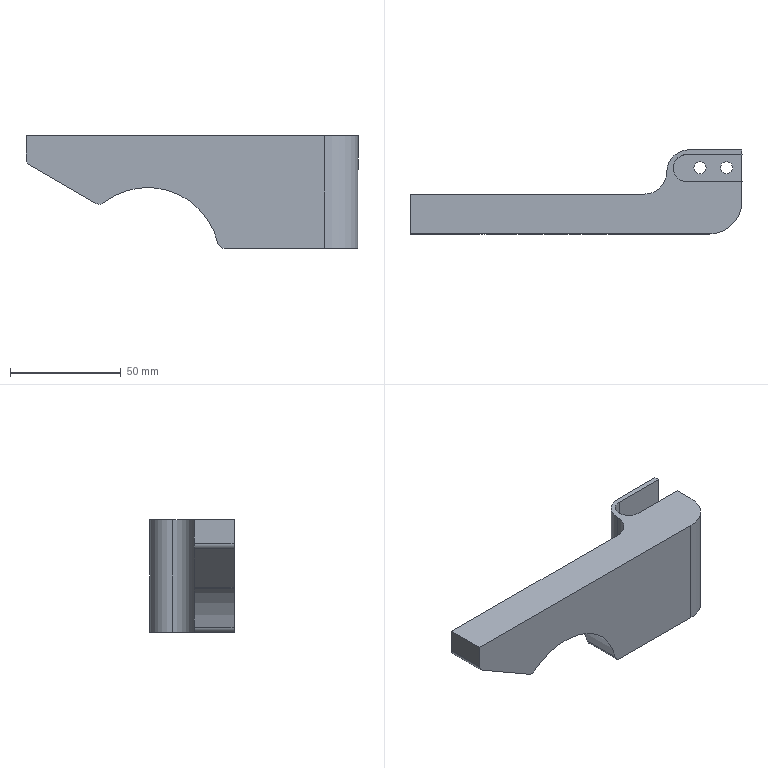Part | NX | 1 solid | 25 faces | box 150 x 38 x 51 mm | volume 119385 mm3 | plane 13 | cylinder 12 | commonest cylinder face diameters 6 x3 5.5 x2 11.5 x2 20 x2 12.2 x1 30 x1
STEP:
#1=CARTESIAN_POINT('',(75.,16.87,0.));
#2=VERTEX_POINT('',#1);
#3=CARTESIAN_POINT('',(50.,16.87,0.));
#4=VERTEX_POINT('',#3);
#5=CARTESIAN_POINT('',(75.,16.87,0.));
#6=DIRECTION('',(-1.,0.,0.));
#7=VECTOR('',#6,1000.);
#8=LINE('',#5,#7);
#9=EDGE_CURVE('',#2,#4,#8,.T.);
#10=ORIENTED_EDGE('',*,*,#9,.F.);
#11=CARTESIAN_POINT('',(75.,19.,0.));
#12=VERTEX_POINT('',#11);
#13=CARTESIAN_POINT('',(75.,-31.,0.));
#14=DIRECTION('',(0.,1.,0.));
#15=VECTOR('',#14,1000.);
#16=LINE('',#13,#15);
#17=EDGE_CURVE('',#2,#12,#16,.T.);
#18=ORIENTED_EDGE('',*,*,#17,.T.);
#19=CARTESIAN_POINT('',(51.,19.,0.));
#20=VERTEX_POINT('',#19);
#21=CARTESIAN_POINT('',(75.,19.,0.));
#22=DIRECTION('',(-1.,0.,0.));
#23=VECTOR('',#22,1000.);
#24=LINE('',#21,#23);
#25=EDGE_CURVE('',#12,#20,#24,.T.);
#26=ORIENTED_EDGE('',*,*,#25,.T.);
#27=CARTESIAN_POINT('',(41.,9.,0.));
#28=VERTEX_POINT('',#27);
#29=CARTESIAN_POINT('',(51.,9.,0.));
#30=DIRECTION('',(0.,0.,1.));
#31=DIRECTION('',(1.,0.,0.));
#32=AXIS2_PLACEMENT_3D('',#29,#30,#31);
#33=CIRCLE('',#32,10.);
#34=EDGE_CURVE('',#20,#28,#33,.T.);
#35=ORIENTED_EDGE('',*,*,#34,.T.);
#36=CARTESIAN_POINT('',(31.,-1.,0.));
#37=VERTEX_POINT('',#36);
#38=CARTESIAN_POINT('',(31.,9.,0.));
#39=DIRECTION('',(0.,0.,-1.));
#40=DIRECTION('',(0.,1.,0.));
#41=AXIS2_PLACEMENT_3D('',#38,#39,#40);
#42=CIRCLE('',#41,10.);
#43=EDGE_CURVE('',#28,#37,#42,.T.);
#44=ORIENTED_EDGE('',*,*,#43,.T.);
#45=CARTESIAN_POINT('',(-75.,-1.,0.));
#46=VERTEX_POINT('',#45);
#47=CARTESIAN_POINT('',(31.,-1.,0.));
#48=DIRECTION('',(-1.,0.,0.));
#49=VECTOR('',#48,1000.);
#50=LINE('',#47,#49);
#51=EDGE_CURVE('',#37,#46,#50,.T.);
#52=ORIENTED_EDGE('',*,*,#51,.T.);
#53=CARTESIAN_POINT('',(-75.,-19.,0.));
#54=VERTEX_POINT('',#53);
#55=CARTESIAN_POINT('',(-75.,-31.,0.));
#56=DIRECTION('',(0.,1.,0.));
#57=VECTOR('',#56,1000.);
#58=LINE('',#55,#57);
#59=EDGE_CURVE('',#46,#54,#58,.F.);
#60=ORIENTED_EDGE('',*,*,#59,.T.);
#61=CARTESIAN_POINT('',(60.,-19.,0.));
#62=VERTEX_POINT('',#61);
#63=CARTESIAN_POINT('',(-75.,-19.,0.));
#64=DIRECTION('',(1.,0.,0.));
#65=VECTOR('',#64,1000.);
#66=LINE('',#63,#65);
#67=EDGE_CURVE('',#54,#62,#66,.T.);
#68=ORIENTED_EDGE('',*,*,#67,.T.);
#69=CARTESIAN_POINT('',(75.,-4.,0.));
#70=VERTEX_POINT('',#69);
#71=CARTESIAN_POINT('',(60.,-4.,0.));
#72=DIRECTION('',(0.,0.,1.));
#73=DIRECTION('',(1.,0.,0.));
#74=AXIS2_PLACEMENT_3D('',#71,#72,#73);
#75=CIRCLE('',#74,15.);
#76=EDGE_CURVE('',#62,#70,#75,.T.);
#77=ORIENTED_EDGE('',*,*,#76,.T.);
#78=CARTESIAN_POINT('',(75.,4.67,0.));
#79=VERTEX_POINT('',#78);
#80=CARTESIAN_POINT('',(75.,-31.,0.));
#81=DIRECTION('',(0.,1.,0.));
#82=VECTOR('',#81,1000.);
#83=LINE('',#80,#82);
#84=EDGE_CURVE('',#70,#79,#83,.T.);
#85=ORIENTED_EDGE('',*,*,#84,.T.);
#86=CARTESIAN_POINT('',(50.,4.67,0.));
#87=VERTEX_POINT('',#86);
#88=CARTESIAN_POINT('',(50.,4.67,0.));
#89=DIRECTION('',(1.,0.,0.));
#90=VECTOR('',#89,1000.);
#91=LINE('',#88,#90);
#92=EDGE_CURVE('',#87,#79,#91,.T.);
#93=ORIENTED_EDGE('',*,*,#92,.F.);
#94=CARTESIAN_POINT('',(50.,10.77,0.));
#95=DIRECTION('',(0.,0.,1.));
#96=DIRECTION('',(1.,0.,0.));
#97=AXIS2_PLACEMENT_3D('',#94,#95,#96);
#98=CIRCLE('',#97,6.1);
#99=EDGE_CURVE('',#4,#87,#98,.T.);
#100=ORIENTED_EDGE('',*,*,#99,.F.);
#101=EDGE_LOOP('',(#10,#18,#26,#35,#44,#52,#60,#68,#77,#85,#93,#100));
#102=FACE_BOUND('',#101,.T.);
#103=CARTESIAN_POINT('',(75.,-31.,0.));
#104=DIRECTION('',(0.,0.,-1.));
#105=DIRECTION('',(0.,1.,0.));
#106=AXIS2_PLACEMENT_3D('',#103,#104,#105);
#107=PLANE('',#106);
#108=ADVANCED_FACE('',(#102),#107,.F.);
#109=CARTESIAN_POINT('',(70.75,10.9,-25.2));
#110=VERTEX_POINT('',#109);
#111=CARTESIAN_POINT('',(68.,10.9,-25.2));
#112=DIRECTION('',(0.,0.,-1.));
#113=DIRECTION('',(1.,0.,0.));
#114=AXIS2_PLACEMENT_3D('',#111,#112,#113);
#115=CIRCLE('',#114,2.75);
#116=EDGE_CURVE('',#110,#110,#115,.F.);
#117=ORIENTED_EDGE('',*,*,#116,.F.);
#118=EDGE_LOOP('',(#117));
#119=FACE_BOUND('',#118,.T.);
#120=CARTESIAN_POINT('',(70.75,10.9,-15.2));
#121=VERTEX_POINT('',#120);
#122=CARTESIAN_POINT('',(68.,10.9,-15.2));
#123=DIRECTION('',(0.,0.,1.));
#124=DIRECTION('',(1.,0.,0.));
#125=AXIS2_PLACEMENT_3D('',#122,#123,#124);
#126=CIRCLE('',#125,2.75);
#127=EDGE_CURVE('',#121,#121,#126,.F.);
#128=ORIENTED_EDGE('',*,*,#127,.F.);
#129=EDGE_LOOP('',(#128));
#130=FACE_BOUND('',#129,.T.);
#131=CARTESIAN_POINT('',(68.,10.9,0.));
#132=DIRECTION('',(0.,0.,-1.));
#133=DIRECTION('',(1.,0.,0.));
#134=AXIS2_PLACEMENT_3D('',#131,#132,#133);
#135=CYLINDRICAL_SURFACE('',#134,2.75);
#136=ADVANCED_FACE('',(#119,#130),#135,.F.);
#137=CARTESIAN_POINT('',(58.75,10.9,-25.2));
#138=VERTEX_POINT('',#137);
#139=CARTESIAN_POINT('',(56.,10.9,-25.2));
#140=DIRECTION('',(0.,0.,-1.));
#141=DIRECTION('',(1.,0.,0.));
#142=AXIS2_PLACEMENT_3D('',#139,#140,#141);
#143=CIRCLE('',#142,2.75);
#144=EDGE_CURVE('',#138,#138,#143,.F.);
#145=ORIENTED_EDGE('',*,*,#144,.F.);
#146=EDGE_LOOP('',(#145));
#147=FACE_BOUND('',#146,.T.);
#148=CARTESIAN_POINT('',(58.75,10.9,-15.2));
#149=VERTEX_POINT('',#148);
#150=CARTESIAN_POINT('',(56.,10.9,-15.2));
#151=DIRECTION('',(0.,0.,1.));
#152=DIRECTION('',(1.,0.,0.));
#153=AXIS2_PLACEMENT_3D('',#150,#151,#152);
#154=CIRCLE('',#153,2.75);
#155=EDGE_CURVE('',#149,#149,#154,.F.);
#156=ORIENTED_EDGE('',*,*,#155,.F.);
#157=EDGE_LOOP('',(#156));
#158=FACE_BOUND('',#157,.T.);
#159=CARTESIAN_POINT('',(56.,10.9,0.));
#160=DIRECTION('',(0.,0.,-1.));
#161=DIRECTION('',(1.,0.,0.));
#162=AXIS2_PLACEMENT_3D('',#159,#160,#161);
#163=CYLINDRICAL_SURFACE('',#162,2.75);
#164=ADVANCED_FACE('',(#147,#158),#163,.F.);
#165=CARTESIAN_POINT('',(-73.5,-19.,-13.246));
#166=VERTEX_POINT('',#165);
#167=CARTESIAN_POINT('',(-73.5,-1.,-13.246));
#168=VERTEX_POINT('',#167);
#169=CARTESIAN_POINT('',(-73.5,-31.,-13.246));
#170=DIRECTION('',(0.,1.,0.));
#171=VECTOR('',#170,1000.);
#172=LINE('',#169,#171);
#173=EDGE_CURVE('',#166,#168,#172,.T.);
#174=ORIENTED_EDGE('',*,*,#173,.F.);
#175=CARTESIAN_POINT('',(-75.,-19.,-10.648));
#176=VERTEX_POINT('',#175);
#177=CARTESIAN_POINT('',(-72.,-19.,-10.648));
#178=DIRECTION('',(0.,1.,0.));
#179=DIRECTION('',(1.,0.,0.));
#180=AXIS2_PLACEMENT_3D('',#177,#178,#179);
#181=CIRCLE('',#180,3.);
#182=EDGE_CURVE('',#166,#176,#181,.T.);
#183=ORIENTED_EDGE('',*,*,#182,.T.);
#184=CARTESIAN_POINT('',(-75.,-1.,-10.648));
#185=VERTEX_POINT('',#184);
#186=CARTESIAN_POINT('',(-75.,-31.,-10.648));
#187=DIRECTION('',(0.,1.,0.));
#188=VECTOR('',#187,1000.);
#189=LINE('',#186,#188);
#190=EDGE_CURVE('',#176,#185,#189,.T.);
#191=ORIENTED_EDGE('',*,*,#190,.T.);
#192=CARTESIAN_POINT('',(-72.,-1.,-10.648));
#193=DIRECTION('',(0.,-1.,0.));
#194=DIRECTION('',(-1.,0.,0.));
#195=AXIS2_PLACEMENT_3D('',#192,#193,#194);
#196=CIRCLE('',#195,3.);
#197=EDGE_CURVE('',#185,#168,#196,.T.);
#198=ORIENTED_EDGE('',*,*,#197,.T.);
#199=EDGE_LOOP('',(#174,#183,#191,#198));
#200=FACE_BOUND('',#199,.T.);
#201=CARTESIAN_POINT('',(-72.,-31.,-10.648));
#202=DIRECTION('',(0.,1.,0.));
#203=DIRECTION('',(1.,0.,0.));
#204=AXIS2_PLACEMENT_3D('',#201,#202,#203);
#205=CYLINDRICAL_SURFACE('',#204,3.);
#206=ADVANCED_FACE('',(#200),#205,.T.);
#207=CARTESIAN_POINT('',(-43.38,-19.,-30.636));
#208=VERTEX_POINT('',#207);
#209=CARTESIAN_POINT('',(-43.38,-1.,-30.636));
#210=VERTEX_POINT('',#209);
#211=CARTESIAN_POINT('',(-43.38,-31.,-30.636));
#212=DIRECTION('',(0.,1.,0.));
#213=VECTOR('',#212,1000.);
#214=LINE('',#211,#213);
#215=EDGE_CURVE('',#208,#210,#214,.T.);
#216=ORIENTED_EDGE('',*,*,#215,.F.);
#217=CARTESIAN_POINT('',(-73.5,-19.,-13.246));
#218=DIRECTION('',(-0.866,0.,0.5));
#219=VECTOR('',#218,1000.);
#220=LINE('',#217,#219);
#221=EDGE_CURVE('',#208,#166,#220,.T.);
#222=ORIENTED_EDGE('',*,*,#221,.T.);
#223=ORIENTED_EDGE('',*,*,#173,.T.);
#224=CARTESIAN_POINT('',(-73.5,-1.,-13.246));
#225=DIRECTION('',(0.866,0.,-0.5));
#226=VECTOR('',#225,1000.);
#227=LINE('',#224,#226);
#228=EDGE_CURVE('',#168,#210,#227,.T.);
#229=ORIENTED_EDGE('',*,*,#228,.T.);
#230=EDGE_LOOP('',(#216,#222,#223,#229));
#231=FACE_BOUND('',#230,.T.);
#232=CARTESIAN_POINT('',(-73.5,-31.,-13.246));
#233=DIRECTION('',(0.5,0.,0.866));
#234=DIRECTION('',(0.866,0.,-0.5));
#235=AXIS2_PLACEMENT_3D('',#232,#233,#234);
#236=PLANE('',#235);
#237=ADVANCED_FACE('',(#231),#236,.F.);
#238=CARTESIAN_POINT('',(-40.031,-19.,-30.401));
#239=VERTEX_POINT('',#238);
#240=CARTESIAN_POINT('',(-40.031,-1.,-30.401));
#241=VERTEX_POINT('',#240);
#242=CARTESIAN_POINT('',(-40.031,-31.,-30.401));
#243=DIRECTION('',(0.,1.,0.));
#244=VECTOR('',#243,1000.);
#245=LINE('',#242,#244);
#246=EDGE_CURVE('',#239,#241,#245,.T.);
#247=ORIENTED_EDGE('',*,*,#246,.F.);
#248=CARTESIAN_POINT('',(-41.88,-19.,-28.038));
#249=DIRECTION('',(0.,1.,0.));
#250=DIRECTION('',(1.,0.,0.));
#251=AXIS2_PLACEMENT_3D('',#248,#249,#250);
#252=CIRCLE('',#251,3.);
#253=EDGE_CURVE('',#239,#208,#252,.T.);
#254=ORIENTED_EDGE('',*,*,#253,.T.);
#255=ORIENTED_EDGE('',*,*,#215,.T.);
#256=CARTESIAN_POINT('',(-41.88,-1.,-28.038));
#257=DIRECTION('',(0.,-1.,0.));
#258=DIRECTION('',(-1.,0.,0.));
#259=AXIS2_PLACEMENT_3D('',#256,#257,#258);
#260=CIRCLE('',#259,3.);
#261=EDGE_CURVE('',#210,#241,#260,.T.);
#262=ORIENTED_EDGE('',*,*,#261,.T.);
#263=EDGE_LOOP('',(#247,#254,#255,#262));
#264=FACE_BOUND('',#263,.T.);
#265=CARTESIAN_POINT('',(-41.88,-31.,-28.038));
#266=DIRECTION('',(0.,1.,0.));
#267=DIRECTION('',(1.,0.,0.));
#268=AXIS2_PLACEMENT_3D('',#265,#266,#267);
#269=CYLINDRICAL_SURFACE('',#268,3.);
#270=ADVANCED_FACE('',(#264),#269,.T.);
#271=CARTESIAN_POINT('',(11.66,-19.,-48.676));
#272=VERTEX_POINT('',#271);
#273=CARTESIAN_POINT('',(11.66,-1.,-48.676));
#274=VERTEX_POINT('',#273);
#275=CARTESIAN_POINT('',(11.66,-31.,-48.676));
#276=DIRECTION('',(0.,1.,0.));
#277=VECTOR('',#276,1000.);
#278=LINE('',#275,#277);
#279=EDGE_CURVE('',#272,#274,#278,.T.);
#280=ORIENTED_EDGE('',*,*,#279,.F.);
#281=CARTESIAN_POINT('',(-20.005,-19.,-55.997));
#282=DIRECTION('',(0.,1.,0.));
#283=DIRECTION('',(1.,0.,0.));
#284=AXIS2_PLACEMENT_3D('',#281,#282,#283);
#285=CIRCLE('',#284,32.5);
#286=EDGE_CURVE('',#272,#239,#285,.F.);
#287=ORIENTED_EDGE('',*,*,#286,.T.);
#288=ORIENTED_EDGE('',*,*,#246,.T.);
#289=CARTESIAN_POINT('',(-20.005,-1.,-55.997));
#290=DIRECTION('',(0.,-1.,0.));
#291=DIRECTION('',(-1.,0.,0.));
#292=AXIS2_PLACEMENT_3D('',#289,#290,#291);
#293=CIRCLE('',#292,32.5);
#294=EDGE_CURVE('',#241,#274,#293,.F.);
#295=ORIENTED_EDGE('',*,*,#294,.T.);
#296=EDGE_LOOP('',(#280,#287,#288,#295));
#297=FACE_BOUND('',#296,.T.);
#298=CARTESIAN_POINT('',(-20.005,-31.,-55.997));
#299=DIRECTION('',(0.,1.,0.));
#300=DIRECTION('',(1.,0.,0.));
#301=AXIS2_PLACEMENT_3D('',#298,#299,#300);
#302=CYLINDRICAL_SURFACE('',#301,32.5);
#303=ADVANCED_FACE('',(#297),#302,.F.);
#304=CARTESIAN_POINT('',(14.583,-19.,-51.));
#305=VERTEX_POINT('',#304);
#306=CARTESIAN_POINT('',(14.583,-1.,-51.));
#307=VERTEX_POINT('',#306);
#308=CARTESIAN_POINT('',(14.583,-31.,-51.));
#309=DIRECTION('',(0.,1.,0.));
#310=VECTOR('',#309,1000.);
#311=LINE('',#308,#310);
#312=EDGE_CURVE('',#305,#307,#311,.T.);
#313=ORIENTED_EDGE('',*,*,#312,.F.);
#314=CARTESIAN_POINT('',(14.583,-19.,-48.));
#315=DIRECTION('',(0.,1.,0.));
#316=DIRECTION('',(1.,0.,0.));
#317=AXIS2_PLACEMENT_3D('',#314,#315,#316);
#318=CIRCLE('',#317,3.);
#319=EDGE_CURVE('',#305,#272,#318,.T.);
#320=ORIENTED_EDGE('',*,*,#319,.T.);
#321=ORIENTED_EDGE('',*,*,#279,.T.);
#322=CARTESIAN_POINT('',(14.583,-1.,-48.));
#323=DIRECTION('',(0.,-1.,0.));
#324=DIRECTION('',(-1.,0.,0.));
#325=AXIS2_PLACEMENT_3D('',#322,#323,#324);
#326=CIRCLE('',#325,3.);
#327=EDGE_CURVE('',#274,#307,#326,.T.);
#328=ORIENTED_EDGE('',*,*,#327,.T.);
#329=EDGE_LOOP('',(#313,#320,#321,#328));
#330=FACE_BOUND('',#329,.T.);
#331=CARTESIAN_POINT('',(14.583,-31.,-48.));
#332=DIRECTION('',(0.,1.,0.));
#333=DIRECTION('',(1.,0.,0.));
#334=AXIS2_PLACEMENT_3D('',#331,#332,#333);
#335=CYLINDRICAL_SURFACE('',#334,3.);
#336=ADVANCED_FACE('',(#330),#335,.T.);
#337=CARTESIAN_POINT('',(51.,19.,-51.));
#338=VERTEX_POINT('',#337);
#339=CARTESIAN_POINT('',(41.,9.,-51.));
#340=VERTEX_POINT('',#339);
#341=CARTESIAN_POINT('',(51.,9.,-51.));
#342=DIRECTION('',(0.,0.,1.));
#343=DIRECTION('',(1.,0.,0.));
#344=AXIS2_PLACEMENT_3D('',#341,#342,#343);
#345=CIRCLE('',#344,10.);
#346=EDGE_CURVE('',#338,#340,#345,.T.);
#347=ORIENTED_EDGE('',*,*,#346,.T.);
#348=CARTESIAN_POINT('',(41.,9.,0.));
#349=DIRECTION('',(0.,0.,-1.));
#350=VECTOR('',#349,1000.);
#351=LINE('',#348,#350);
#352=EDGE_CURVE('',#28,#340,#351,.T.);
#353=ORIENTED_EDGE('',*,*,#352,.F.);
#354=ORIENTED_EDGE('',*,*,#34,.F.);
#355=CARTESIAN_POINT('',(51.,19.,0.));
#356=DIRECTION('',(0.,0.,-1.));
#357=VECTOR('',#356,1000.);
#358=LINE('',#355,#357);
#359=EDGE_CURVE('',#20,#338,#358,.T.);
#360=ORIENTED_EDGE('',*,*,#359,.T.);
#361=EDGE_LOOP('',(#347,#353,#354,#360));
#362=FACE_BOUND('',#361,.T.);
#363=CARTESIAN_POINT('',(51.,9.,0.));
#364=DIRECTION('',(0.,0.,-1.));
#365=DIRECTION('',(1.,0.,0.));
#366=AXIS2_PLACEMENT_3D('',#363,#364,#365);
#367=CYLINDRICAL_SURFACE('',#366,10.);
#368=ADVANCED_FACE('',(#362),#367,.T.);
#369=ORIENTED_EDGE('',*,*,#197,.F.);
#370=CARTESIAN_POINT('',(-75.,-1.,0.));
#371=DIRECTION('',(0.,0.,-1.));
#372=VECTOR('',#371,1000.);
#373=LINE('',#370,#372);
#374=EDGE_CURVE('',#46,#185,#373,.T.);
#375=ORIENTED_EDGE('',*,*,#374,.F.);
#376=ORIENTED_EDGE('',*,*,#51,.F.);
#377=CARTESIAN_POINT('',(31.,-1.,-51.));
#378=VERTEX_POINT('',#377);
#379=CARTESIAN_POINT('',(31.,-1.,0.));
#380=DIRECTION('',(0.,0.,-1.));
#381=VECTOR('',#380,1000.);
#382=LINE('',#379,#381);
#383=EDGE_CURVE('',#37,#378,#382,.T.);
#384=ORIENTED_EDGE('',*,*,#383,.T.);
#385=CARTESIAN_POINT('',(31.,-1.,-51.));
#386=DIRECTION('',(-1.,0.,0.));
#387=VECTOR('',#386,1000.);
#388=LINE('',#385,#387);
#389=EDGE_CURVE('',#378,#307,#388,.T.);
#390=ORIENTED_EDGE('',*,*,#389,.T.);
#391=ORIENTED_EDGE('',*,*,#327,.F.);
#392=ORIENTED_EDGE('',*,*,#294,.F.);
#393=ORIENTED_EDGE('',*,*,#261,.F.);
#394=ORIENTED_EDGE('',*,*,#228,.F.);
#395=EDGE_LOOP('',(#369,#375,#376,#384,#390,#391,#392,#393,#394));
#396=FACE_BOUND('',#395,.T.);
#397=CARTESIAN_POINT('',(31.,-1.,0.));
#398=DIRECTION('',(0.,-1.,0.));
#399=DIRECTION('',(0.,0.,-1.));
#400=AXIS2_PLACEMENT_3D('',#397,#398,#399);
#401=PLANE('',#400);
#402=ADVANCED_FACE('',(#396),#401,.F.);
#403=CARTESIAN_POINT('',(31.,9.,-51.));
#404=DIRECTION('',(0.,0.,1.));
#405=DIRECTION('',(0.,-1.,0.));
#406=AXIS2_PLACEMENT_3D('',#403,#404,#405);
#407=CIRCLE('',#406,10.);
#408=EDGE_CURVE('',#340,#378,#407,.F.);
#409=ORIENTED_EDGE('',*,*,#408,.T.);
#410=ORIENTED_EDGE('',*,*,#383,.F.);
#411=ORIENTED_EDGE('',*,*,#43,.F.);
#412=ORIENTED_EDGE('',*,*,#352,.T.);
#413=EDGE_LOOP('',(#409,#410,#411,#412));
#414=FACE_BOUND('',#413,.T.);
#415=CARTESIAN_POINT('',(31.,9.,0.));
#416=DIRECTION('',(0.,0.,-1.));
#417=DIRECTION('',(1.,0.,0.));
#418=AXIS2_PLACEMENT_3D('',#415,#416,#417);
#419=CYLINDRICAL_SURFACE('',#418,10.);
#420=ADVANCED_FACE('',(#414),#419,.F.);
#421=CARTESIAN_POINT('',(60.,-19.,-51.));
#422=VERTEX_POINT('',#421);
#423=CARTESIAN_POINT('',(75.,-4.,-51.));
#424=VERTEX_POINT('',#423);
#425=CARTESIAN_POINT('',(60.,-4.,-51.));
#426=DIRECTION('',(0.,0.,1.));
#427=DIRECTION('',(1.,0.,0.));
#428=AXIS2_PLACEMENT_3D('',#425,#426,#427);
#429=CIRCLE('',#428,15.);
#430=EDGE_CURVE('',#422,#424,#429,.T.);
#431=ORIENTED_EDGE('',*,*,#430,.T.);
#432=CARTESIAN_POINT('',(75.,-4.,0.));
#433=DIRECTION('',(0.,0.,-1.));
#434=VECTOR('',#433,1000.);
#435=LINE('',#432,#434);
#436=EDGE_CURVE('',#70,#424,#435,.T.);
#437=ORIENTED_EDGE('',*,*,#436,.F.);
#438=ORIENTED_EDGE('',*,*,#76,.F.);
#439=CARTESIAN_POINT('',(60.,-19.,0.));
#440=DIRECTION('',(0.,0.,-1.));
#441=VECTOR('',#440,1000.);
#442=LINE('',#439,#441);
#443=EDGE_CURVE('',#62,#422,#442,.T.);
#444=ORIENTED_EDGE('',*,*,#443,.T.);
#445=EDGE_LOOP('',(#431,#437,#438,#444));
#446=FACE_BOUND('',#445,.T.);
#447=CARTESIAN_POINT('',(60.,-4.,0.));
#448=DIRECTION('',(0.,0.,-1.));
#449=DIRECTION('',(1.,0.,0.));
#450=AXIS2_PLACEMENT_3D('',#447,#448,#449);
#451=CYLINDRICAL_SURFACE('',#450,15.);
#452=ADVANCED_FACE('',(#446),#451,.T.);
#453=ORIENTED_EDGE('',*,*,#182,.F.);
#454=ORIENTED_EDGE('',*,*,#221,.F.);
#455=ORIENTED_EDGE('',*,*,#253,.F.);
#456=ORIENTED_EDGE('',*,*,#286,.F.);
#457=ORIENTED_EDGE('',*,*,#319,.F.);
#458=CARTESIAN_POINT('',(-75.,-19.,-51.));
#459=DIRECTION('',(1.,0.,0.));
#460=VECTOR('',#459,1000.);
#461=LINE('',#458,#460);
#462=EDGE_CURVE('',#305,#422,#461,.T.);
#463=ORIENTED_EDGE('',*,*,#462,.T.);
#464=ORIENTED_EDGE('',*,*,#443,.F.);
#465=ORIENTED_EDGE('',*,*,#67,.F.);
#466=CARTESIAN_POINT('',(-75.,-19.,0.));
#467=DIRECTION('',(0.,0.,-1.));
#468=VECTOR('',#467,1000.);
#469=LINE('',#466,#468);
#470=EDGE_CURVE('',#54,#176,#469,.T.);
#471=ORIENTED_EDGE('',*,*,#470,.T.);
#472=EDGE_LOOP('',(#453,#454,#455,#456,#457,#463,#464,#465,#471));
#473=FACE_BOUND('',#472,.T.);
#474=CARTESIAN_POINT('',(-75.,-19.,0.));
#475=DIRECTION('',(0.,1.,0.));
#476=DIRECTION('',(0.,0.,1.));
#477=AXIS2_PLACEMENT_3D('',#474,#475,#476);
#478=PLANE('',#477);
#479=ADVANCED_FACE('',(#473),#478,.F.);
#480=CARTESIAN_POINT('',(73.75,10.9,-25.2));
#481=VERTEX_POINT('',#480);
#482=CARTESIAN_POINT('',(68.,10.9,-25.2));
#483=DIRECTION('',(0.,0.,-1.));
#484=DIRECTION('',(1.,0.,0.));
#485=AXIS2_PLACEMENT_3D('',#482,#483,#484);
#486=CIRCLE('',#485,5.75);
#487=EDGE_CURVE('',#481,#481,#486,.F.);
#488=ORIENTED_EDGE('',*,*,#487,.F.);
#489=EDGE_LOOP('',(#488));
#490=FACE_BOUND('',#489,.T.);
#491=ORIENTED_EDGE('',*,*,#116,.T.);
#492=EDGE_LOOP('',(#491));
#493=FACE_BOUND('',#492,.T.);
#494=CARTESIAN_POINT('',(68.,10.9,-25.2));
#495=DIRECTION('',(0.,0.,-1.));
#496=DIRECTION('',(1.,0.,0.));
#497=AXIS2_PLACEMENT_3D('',#494,#495,#496);
#498=PLANE('',#497);
#499=ADVANCED_FACE('',(#490,#493),#498,.T.);
#500=ORIENTED_EDGE('',*,*,#487,.T.);
#501=EDGE_LOOP('',(#500));
#502=FACE_BOUND('',#501,.T.);
#503=CARTESIAN_POINT('',(68.,5.15,-51.));
#504=VERTEX_POINT('',#503);
#505=CARTESIAN_POINT('',(68.,10.9,-51.));
#506=DIRECTION('',(0.,0.,1.));
#507=DIRECTION('',(0.,-1.,0.));
#508=AXIS2_PLACEMENT_3D('',#505,#506,#507);
#509=CIRCLE('',#508,5.75);
#510=EDGE_CURVE('',#504,#504,#509,.F.);
#511=ORIENTED_EDGE('',*,*,#510,.T.);
#512=EDGE_LOOP('',(#511));
#513=FACE_BOUND('',#512,.T.);
#514=CARTESIAN_POINT('',(68.,10.9,-25.2));
#515=DIRECTION('',(0.,0.,-1.));
#516=DIRECTION('',(1.,0.,0.));
#517=AXIS2_PLACEMENT_3D('',#514,#515,#516);
#518=CYLINDRICAL_SURFACE('',#517,5.75);
#519=ADVANCED_FACE('',(#502,#513),#518,.F.);
#520=CARTESIAN_POINT('',(61.75,10.9,-25.2));
#521=VERTEX_POINT('',#520);
#522=CARTESIAN_POINT('',(56.,10.9,-25.2));
#523=DIRECTION('',(0.,0.,-1.));
#524=DIRECTION('',(1.,0.,0.));
#525=AXIS2_PLACEMENT_3D('',#522,#523,#524);
#526=CIRCLE('',#525,5.75);
#527=EDGE_CURVE('',#521,#521,#526,.F.);
#528=ORIENTED_EDGE('',*,*,#527,.T.);
#529=EDGE_LOOP('',(#528));
#530=FACE_BOUND('',#529,.T.);
#531=CARTESIAN_POINT('',(56.,5.15,-51.));
#532=VERTEX_POINT('',#531);
#533=CARTESIAN_POINT('',(56.,10.9,-51.));
#534=DIRECTION('',(0.,0.,1.));
#535=DIRECTION('',(0.,-1.,0.));
#536=AXIS2_PLACEMENT_3D('',#533,#534,#535);
#537=CIRCLE('',#536,5.75);
#538=EDGE_CURVE('',#532,#532,#537,.F.);
#539=ORIENTED_EDGE('',*,*,#538,.T.);
#540=EDGE_LOOP('',(#539));
#541=FACE_BOUND('',#540,.T.);
#542=CARTESIAN_POINT('',(56.,10.9,-25.2));
#543=DIRECTION('',(0.,0.,-1.));
#544=DIRECTION('',(1.,0.,0.));
#545=AXIS2_PLACEMENT_3D('',#542,#543,#544);
#546=CYLINDRICAL_SURFACE('',#545,5.75);
#547=ADVANCED_FACE('',(#530,#541),#546,.F.);
#548=ORIENTED_EDGE('',*,*,#527,.F.);
#549=EDGE_LOOP('',(#548));
#550=FACE_BOUND('',#549,.T.);
#551=ORIENTED_EDGE('',*,*,#144,.T.);
#552=EDGE_LOOP('',(#551));
#553=FACE_BOUND('',#552,.T.);
#554=CARTESIAN_POINT('',(56.,10.9,-25.2));
#555=DIRECTION('',(0.,0.,-1.));
#556=DIRECTION('',(1.,0.,0.));
#557=AXIS2_PLACEMENT_3D('',#554,#555,#556);
#558=PLANE('',#557);
#559=ADVANCED_FACE('',(#550,#553),#558,.T.);
#560=ORIENTED_EDGE('',*,*,#510,.F.);
#561=EDGE_LOOP('',(#560));
#562=FACE_BOUND('',#561,.T.);
#563=ORIENTED_EDGE('',*,*,#538,.F.);
#564=EDGE_LOOP('',(#563));
#565=FACE_BOUND('',#564,.T.);
#566=ORIENTED_EDGE('',*,*,#389,.F.);
#567=ORIENTED_EDGE('',*,*,#408,.F.);
#568=ORIENTED_EDGE('',*,*,#346,.F.);
#569=CARTESIAN_POINT('',(75.,19.,-51.));
#570=VERTEX_POINT('',#569);
#571=CARTESIAN_POINT('',(14.583,19.,-51.));
#572=DIRECTION('',(1.,0.,0.));
#573=VECTOR('',#572,1000.);
#574=LINE('',#571,#573);
#575=EDGE_CURVE('',#570,#338,#574,.F.);
#576=ORIENTED_EDGE('',*,*,#575,.F.);
#577=CARTESIAN_POINT('',(75.,-31.,-51.));
#578=DIRECTION('',(0.,1.,0.));
#579=VECTOR('',#578,1000.);
#580=LINE('',#577,#579);
#581=EDGE_CURVE('',#424,#570,#580,.T.);
#582=ORIENTED_EDGE('',*,*,#581,.F.);
#583=ORIENTED_EDGE('',*,*,#430,.F.);
#584=ORIENTED_EDGE('',*,*,#462,.F.);
#585=ORIENTED_EDGE('',*,*,#312,.T.);
#586=EDGE_LOOP('',(#566,#567,#568,#576,#582,#583,#584,#585));
#587=FACE_BOUND('',#586,.T.);
#588=CARTESIAN_POINT('',(14.583,-31.,-51.));
#589=DIRECTION('',(0.,0.,1.));
#590=DIRECTION('',(0.,-1.,0.));
#591=AXIS2_PLACEMENT_3D('',#588,#589,#590);
#592=PLANE('',#591);
#593=ADVANCED_FACE('',(#562,#565,#587),#592,.F.);
#594=ORIENTED_EDGE('',*,*,#359,.F.);
#595=ORIENTED_EDGE('',*,*,#25,.F.);
#596=CARTESIAN_POINT('',(75.,19.,-51.));
#597=DIRECTION('',(0.,0.,1.));
#598=VECTOR('',#597,1000.);
#599=LINE('',#596,#598);
#600=EDGE_CURVE('',#12,#570,#599,.F.);
#601=ORIENTED_EDGE('',*,*,#600,.T.);
#602=ORIENTED_EDGE('',*,*,#575,.T.);
#603=EDGE_LOOP('',(#594,#595,#601,#602));
#604=FACE_BOUND('',#603,.T.);
#605=CARTESIAN_POINT('',(-72.,19.,-10.648));
#606=DIRECTION('',(0.,-1.,0.));
#607=DIRECTION('',(-1.,0.,0.));
#608=AXIS2_PLACEMENT_3D('',#605,#606,#607);
#609=PLANE('',#608);
#610=ADVANCED_FACE('',(#604),#609,.F.);
#611=ORIENTED_EDGE('',*,*,#470,.F.);
#612=ORIENTED_EDGE('',*,*,#59,.F.);
#613=ORIENTED_EDGE('',*,*,#374,.T.);
#614=ORIENTED_EDGE('',*,*,#190,.F.);
#615=EDGE_LOOP('',(#611,#612,#613,#614));
#616=FACE_BOUND('',#615,.T.);
#617=CARTESIAN_POINT('',(-75.,-31.,0.));
#618=DIRECTION('',(1.,0.,0.));
#619=DIRECTION('',(0.,0.,-1.));
#620=AXIS2_PLACEMENT_3D('',#617,#618,#619);
#621=PLANE('',#620);
#622=ADVANCED_FACE('',(#616),#621,.F.);
#623=CARTESIAN_POINT('',(75.,4.67,-15.2));
#624=VERTEX_POINT('',#623);
#625=CARTESIAN_POINT('',(75.,16.87,-15.2));
#626=VERTEX_POINT('',#625);
#627=CARTESIAN_POINT('',(75.,4.67,-15.2));
#628=DIRECTION('',(0.,1.,0.));
#629=VECTOR('',#628,1000.);
#630=LINE('',#627,#629);
#631=EDGE_CURVE('',#624,#626,#630,.T.);
#632=ORIENTED_EDGE('',*,*,#631,.F.);
#633=CARTESIAN_POINT('',(75.,4.67,-15.2));
#634=DIRECTION('',(0.,0.,1.));
#635=VECTOR('',#634,1000.);
#636=LINE('',#633,#635);
#637=EDGE_CURVE('',#624,#79,#636,.T.);
#638=ORIENTED_EDGE('',*,*,#637,.T.);
#639=ORIENTED_EDGE('',*,*,#84,.F.);
#640=ORIENTED_EDGE('',*,*,#436,.T.);
#641=ORIENTED_EDGE('',*,*,#581,.T.);
#642=ORIENTED_EDGE('',*,*,#600,.F.);
#643=ORIENTED_EDGE('',*,*,#17,.F.);
#644=CARTESIAN_POINT('',(75.,16.87,-15.2));
#645=DIRECTION('',(0.,0.,1.));
#646=VECTOR('',#645,1000.);
#647=LINE('',#644,#646);
#648=EDGE_CURVE('',#626,#2,#647,.T.);
#649=ORIENTED_EDGE('',*,*,#648,.F.);
#650=EDGE_LOOP('',(#632,#638,#639,#640,#641,#642,#643,#649));
#651=FACE_BOUND('',#650,.T.);
#652=CARTESIAN_POINT('',(75.,-31.,-51.));
#653=DIRECTION('',(-1.,0.,0.));
#654=DIRECTION('',(0.,1.,0.));
#655=AXIS2_PLACEMENT_3D('',#652,#653,#654);
#656=PLANE('',#655);
#657=ADVANCED_FACE('',(#651),#656,.F.);
#658=CARTESIAN_POINT('',(50.,16.87,-15.2));
#659=VERTEX_POINT('',#658);
#660=CARTESIAN_POINT('',(75.,16.87,-15.2));
#661=DIRECTION('',(-1.,0.,0.));
#662=VECTOR('',#661,1000.);
#663=LINE('',#660,#662);
#664=EDGE_CURVE('',#659,#626,#663,.F.);
#665=ORIENTED_EDGE('',*,*,#664,.F.);
#666=CARTESIAN_POINT('',(50.,4.67,-15.2));
#667=VERTEX_POINT('',#666);
#668=CARTESIAN_POINT('',(50.,10.77,-15.2));
#669=DIRECTION('',(0.,0.,1.));
#670=DIRECTION('',(1.,0.,0.));
#671=AXIS2_PLACEMENT_3D('',#668,#669,#670);
#672=CIRCLE('',#671,6.1);
#673=EDGE_CURVE('',#667,#659,#672,.F.);
#674=ORIENTED_EDGE('',*,*,#673,.F.);
#675=CARTESIAN_POINT('',(50.,4.67,-15.2));
#676=DIRECTION('',(1.,0.,0.));
#677=VECTOR('',#676,1000.);
#678=LINE('',#675,#677);
#679=EDGE_CURVE('',#624,#667,#678,.F.);
#680=ORIENTED_EDGE('',*,*,#679,.F.);
#681=ORIENTED_EDGE('',*,*,#631,.T.);
#682=EDGE_LOOP('',(#665,#674,#680,#681));
#683=FACE_BOUND('',#682,.T.);
#684=ORIENTED_EDGE('',*,*,#155,.T.);
#685=EDGE_LOOP('',(#684));
#686=FACE_BOUND('',#685,.T.);
#687=ORIENTED_EDGE('',*,*,#127,.T.);
#688=EDGE_LOOP('',(#687));
#689=FACE_BOUND('',#688,.T.);
#690=CARTESIAN_POINT('',(50.,10.77,-15.2));
#691=DIRECTION('',(0.,0.,1.));
#692=DIRECTION('',(1.,0.,0.));
#693=AXIS2_PLACEMENT_3D('',#690,#691,#692);
#694=PLANE('',#693);
#695=ADVANCED_FACE('',(#683,#686,#689),#694,.T.);
#696=ORIENTED_EDGE('',*,*,#9,.T.);
#697=CARTESIAN_POINT('',(50.,16.87,-15.2));
#698=DIRECTION('',(0.,0.,1.));
#699=VECTOR('',#698,1000.);
#700=LINE('',#697,#699);
#701=EDGE_CURVE('',#4,#659,#700,.F.);
#702=ORIENTED_EDGE('',*,*,#701,.T.);
#703=ORIENTED_EDGE('',*,*,#664,.T.);
#704=ORIENTED_EDGE('',*,*,#648,.T.);
#705=EDGE_LOOP('',(#696,#702,#703,#704));
#706=FACE_BOUND('',#705,.T.);
#707=CARTESIAN_POINT('',(75.,16.87,-15.2));
#708=DIRECTION('',(0.,1.,0.));
#709=DIRECTION('',(0.,0.,1.));
#710=AXIS2_PLACEMENT_3D('',#707,#708,#709);
#711=PLANE('',#710);
#712=ADVANCED_FACE('',(#706),#711,.F.);
#713=ORIENTED_EDGE('',*,*,#99,.T.);
#714=CARTESIAN_POINT('',(50.,4.67,-15.2));
#715=DIRECTION('',(0.,0.,1.));
#716=VECTOR('',#715,1000.);
#717=LINE('',#714,#716);
#718=EDGE_CURVE('',#87,#667,#717,.F.);
#719=ORIENTED_EDGE('',*,*,#718,.T.);
#720=ORIENTED_EDGE('',*,*,#673,.T.);
#721=ORIENTED_EDGE('',*,*,#701,.F.);
#722=EDGE_LOOP('',(#713,#719,#720,#721));
#723=FACE_BOUND('',#722,.T.);
#724=CARTESIAN_POINT('',(50.,10.77,-15.2));
#725=DIRECTION('',(0.,0.,1.));
#726=DIRECTION('',(1.,0.,0.));
#727=AXIS2_PLACEMENT_3D('',#724,#725,#726);
#728=CYLINDRICAL_SURFACE('',#727,6.1);
#729=ADVANCED_FACE('',(#723),#728,.F.);
#730=ORIENTED_EDGE('',*,*,#92,.T.);
#731=ORIENTED_EDGE('',*,*,#637,.F.);
#732=ORIENTED_EDGE('',*,*,#679,.T.);
#733=ORIENTED_EDGE('',*,*,#718,.F.);
#734=EDGE_LOOP('',(#730,#731,#732,#733));
#735=FACE_BOUND('',#734,.T.);
#736=CARTESIAN_POINT('',(50.,4.67,-15.2));
#737=DIRECTION('',(0.,-1.,0.));
#738=DIRECTION('',(0.,0.,-1.));
#739=AXIS2_PLACEMENT_3D('',#736,#737,#738);
#740=PLANE('',#739);
#741=ADVANCED_FACE('',(#735),#740,.F.);
#742=CLOSED_SHELL('',(#108,#136,#164,#206,#237,#270,#303,#336,#368,#402,#420,#452,#479,#499,#519,#547,#559,#593,#610,#622,#657,#695,#712,#729,#741));
#743=MANIFOLD_SOLID_BREP('',#742);
#744=(LENGTH_UNIT()NAMED_UNIT(*)SI_UNIT(.MILLI.,.METRE.));
#745=UNCERTAINTY_MEASURE_WITH_UNIT(LENGTH_MEASURE(0.00001),#744,'','');
#746=(NAMED_UNIT(*)PLANE_ANGLE_UNIT()SI_UNIT($,.RADIAN.));
#747=(NAMED_UNIT(*)SI_UNIT($,.STERADIAN.)SOLID_ANGLE_UNIT());
#748=(GEOMETRIC_REPRESENTATION_CONTEXT(3)GLOBAL_UNCERTAINTY_ASSIGNED_CONTEXT((#745))GLOBAL_UNIT_ASSIGNED_CONTEXT((#744,#746,#747))REPRESENTATION_CONTEXT('',''));
#749=ADVANCED_BREP_SHAPE_REPRESENTATION('',(#743),#748);